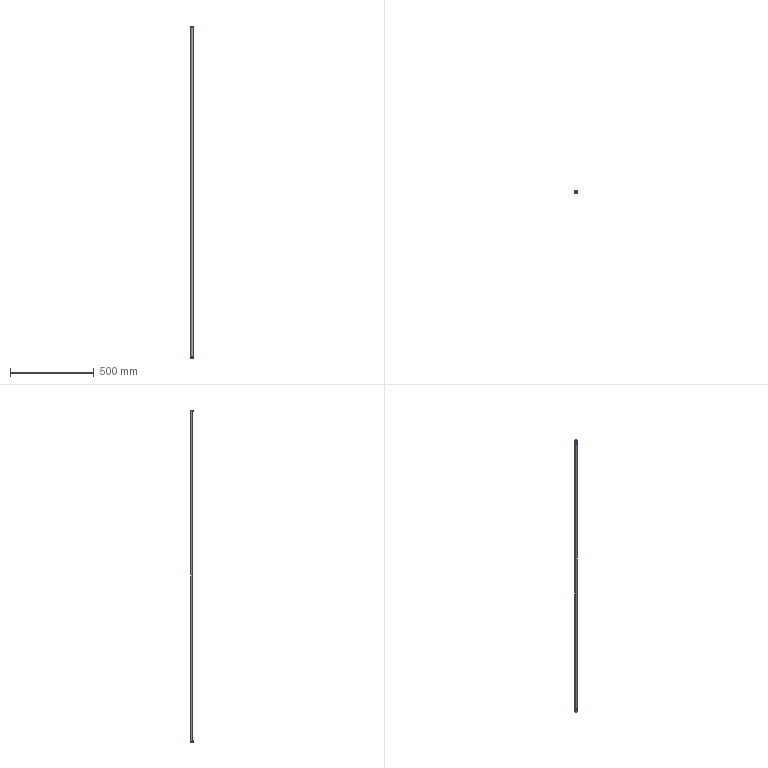Part | STEP file | X77-02003 | 1 solid | 32 faces | box 16 x 16 x 1981 mm | volume 394354 mm3 | plane 12 | cylinder 10 | cone 10 | commonest cylinder face diameters 8.8 x4 10 x4 16 x2
STEP:
#1=CARTESIAN_POINT('',(264.017,-37.994,1961.));
#2=VERTEX_POINT('',#1);
#3=CARTESIAN_POINT('',(274.017,-37.994,1961.));
#4=VERTEX_POINT('',#3);
#5=CARTESIAN_POINT('',(269.017,-37.994,1961.));
#6=DIRECTION('',(0.,0.,1.));
#7=DIRECTION('',(1.,0.,0.));
#8=AXIS2_PLACEMENT_3D('',#5,#6,#7);
#9=CIRCLE('',#8,5.);
#10=EDGE_CURVE('',#2,#4,#9,.T.);
#11=ORIENTED_EDGE('',*,*,#10,.F.);
#12=CARTESIAN_POINT('',(264.017,-37.994,1981.));
#13=VERTEX_POINT('',#12);
#14=CARTESIAN_POINT('',(264.017,-37.994,1981.));
#15=DIRECTION('',(0.,0.,1.));
#16=VECTOR('',#15,1000.);
#17=LINE('',#14,#16);
#18=EDGE_CURVE('',#2,#13,#17,.T.);
#19=ORIENTED_EDGE('',*,*,#18,.T.);
#20=CARTESIAN_POINT('',(274.017,-37.994,1981.));
#21=VERTEX_POINT('',#20);
#22=CARTESIAN_POINT('',(269.017,-37.994,1981.));
#23=DIRECTION('',(0.,0.,1.));
#24=DIRECTION('',(1.,0.,0.));
#25=AXIS2_PLACEMENT_3D('',#22,#23,#24);
#26=CIRCLE('',#25,5.);
#27=EDGE_CURVE('',#13,#21,#26,.T.);
#28=ORIENTED_EDGE('',*,*,#27,.T.);
#29=CARTESIAN_POINT('',(274.017,-37.994,1981.));
#30=DIRECTION('',(0.,0.,1.));
#31=VECTOR('',#30,1000.);
#32=LINE('',#29,#31);
#33=EDGE_CURVE('',#4,#21,#32,.T.);
#34=ORIENTED_EDGE('',*,*,#33,.F.);
#35=EDGE_LOOP('',(#11,#19,#28,#34));
#36=FACE_OUTER_BOUND('',#35,.T.);
#37=CARTESIAN_POINT('',(269.017,-37.994,1981.));
#38=DIRECTION('',(0.,0.,1.));
#39=DIRECTION('',(1.,0.,0.));
#40=AXIS2_PLACEMENT_3D('',#37,#38,#39);
#41=CYLINDRICAL_SURFACE('',#40,5.);
#42=ADVANCED_FACE('',(#36),#41,.F.);
#43=CARTESIAN_POINT('',(264.617,-37.994,1957.25));
#44=VERTEX_POINT('',#43);
#45=CARTESIAN_POINT('',(273.417,-37.994,1957.25));
#46=VERTEX_POINT('',#45);
#47=CARTESIAN_POINT('',(269.017,-37.994,1957.25));
#48=DIRECTION('',(0.,0.,1.));
#49=DIRECTION('',(1.,0.,0.));
#50=AXIS2_PLACEMENT_3D('',#47,#48,#49);
#51=CIRCLE('',#50,4.4);
#52=EDGE_CURVE('',#44,#46,#51,.T.);
#53=ORIENTED_EDGE('',*,*,#52,.F.);
#54=CARTESIAN_POINT('',(264.617,-37.994,1961.));
#55=VERTEX_POINT('',#54);
#56=CARTESIAN_POINT('',(264.617,-37.994,1981.));
#57=DIRECTION('',(0.,0.,1.));
#58=VECTOR('',#57,1000.);
#59=LINE('',#56,#58);
#60=EDGE_CURVE('',#44,#55,#59,.T.);
#61=ORIENTED_EDGE('',*,*,#60,.T.);
#62=CARTESIAN_POINT('',(273.417,-37.994,1961.));
#63=VERTEX_POINT('',#62);
#64=CARTESIAN_POINT('',(269.017,-37.994,1961.));
#65=DIRECTION('',(0.,0.,1.));
#66=DIRECTION('',(1.,0.,0.));
#67=AXIS2_PLACEMENT_3D('',#64,#65,#66);
#68=CIRCLE('',#67,4.4);
#69=EDGE_CURVE('',#55,#63,#68,.T.);
#70=ORIENTED_EDGE('',*,*,#69,.T.);
#71=CARTESIAN_POINT('',(273.417,-37.994,1981.));
#72=DIRECTION('',(0.,0.,1.));
#73=VECTOR('',#72,1000.);
#74=LINE('',#71,#73);
#75=EDGE_CURVE('',#46,#63,#74,.T.);
#76=ORIENTED_EDGE('',*,*,#75,.F.);
#77=EDGE_LOOP('',(#53,#61,#70,#76));
#78=FACE_OUTER_BOUND('',#77,.T.);
#79=CARTESIAN_POINT('',(269.017,-37.994,1981.));
#80=DIRECTION('',(0.,0.,1.));
#81=DIRECTION('',(1.,0.,0.));
#82=AXIS2_PLACEMENT_3D('',#79,#80,#81);
#83=CYLINDRICAL_SURFACE('',#82,4.4);
#84=ADVANCED_FACE('',(#78),#83,.F.);
#85=CARTESIAN_POINT('',(269.017,-37.994,1954.606));
#86=VERTEX_POINT('',#85);
#87=CARTESIAN_POINT('',(273.417,-37.994,1957.25));
#88=DIRECTION('',(0.8572,0.,0.515));
#89=VECTOR('',#88,1000.);
#90=LINE('',#87,#89);
#91=EDGE_CURVE('',#86,#46,#90,.T.);
#92=ORIENTED_EDGE('',*,*,#91,.F.);
#93=CARTESIAN_POINT('',(264.617,-37.994,1957.25));
#94=DIRECTION('',(-0.8572,0.,0.515));
#95=VECTOR('',#94,1000.);
#96=LINE('',#93,#95);
#97=EDGE_CURVE('',#86,#44,#96,.T.);
#98=ORIENTED_EDGE('',*,*,#97,.T.);
#99=ORIENTED_EDGE('',*,*,#52,.T.);
#100=EDGE_LOOP('',(#92,#98,#99));
#101=FACE_OUTER_BOUND('',#100,.T.);
#102=CARTESIAN_POINT('',(269.017,-37.994,1957.25));
#103=DIRECTION('',(0.,0.,1.));
#104=DIRECTION('',(1.,0.,0.));
#105=AXIS2_PLACEMENT_3D('',#102,#103,#104);
#106=CONICAL_SURFACE('',#105,4.4,1.03);
#107=ADVANCED_FACE('',(#101),#106,.F.);
#108=CARTESIAN_POINT('',(274.017,-37.994,20.));
#109=VERTEX_POINT('',#108);
#110=CARTESIAN_POINT('',(264.017,-37.994,20.));
#111=VERTEX_POINT('',#110);
#112=CARTESIAN_POINT('',(269.017,-37.994,20.));
#113=DIRECTION('',(0.,0.,-1.));
#114=DIRECTION('',(-1.,0.,0.));
#115=AXIS2_PLACEMENT_3D('',#112,#113,#114);
#116=CIRCLE('',#115,5.);
#117=EDGE_CURVE('',#109,#111,#116,.T.);
#118=ORIENTED_EDGE('',*,*,#117,.F.);
#119=CARTESIAN_POINT('',(274.017,-37.994,0.));
#120=VERTEX_POINT('',#119);
#121=CARTESIAN_POINT('',(274.017,-37.994,0.));
#122=DIRECTION('',(0.,0.,-1.));
#123=VECTOR('',#122,1000.);
#124=LINE('',#121,#123);
#125=EDGE_CURVE('',#109,#120,#124,.T.);
#126=ORIENTED_EDGE('',*,*,#125,.T.);
#127=CARTESIAN_POINT('',(264.017,-37.994,0.));
#128=VERTEX_POINT('',#127);
#129=CARTESIAN_POINT('',(269.017,-37.994,0.));
#130=DIRECTION('',(0.,0.,-1.));
#131=DIRECTION('',(-1.,0.,0.));
#132=AXIS2_PLACEMENT_3D('',#129,#130,#131);
#133=CIRCLE('',#132,5.);
#134=EDGE_CURVE('',#120,#128,#133,.T.);
#135=ORIENTED_EDGE('',*,*,#134,.T.);
#136=CARTESIAN_POINT('',(264.017,-37.994,0.));
#137=DIRECTION('',(0.,0.,-1.));
#138=VECTOR('',#137,1000.);
#139=LINE('',#136,#138);
#140=EDGE_CURVE('',#111,#128,#139,.T.);
#141=ORIENTED_EDGE('',*,*,#140,.F.);
#142=EDGE_LOOP('',(#118,#126,#135,#141));
#143=FACE_OUTER_BOUND('',#142,.T.);
#144=CARTESIAN_POINT('',(269.017,-37.994,0.));
#145=DIRECTION('',(0.,0.,-1.));
#146=DIRECTION('',(-1.,0.,0.));
#147=AXIS2_PLACEMENT_3D('',#144,#145,#146);
#148=CYLINDRICAL_SURFACE('',#147,5.);
#149=ADVANCED_FACE('',(#143),#148,.F.);
#150=CARTESIAN_POINT('',(273.417,-37.994,23.75));
#151=VERTEX_POINT('',#150);
#152=CARTESIAN_POINT('',(264.617,-37.994,23.75));
#153=VERTEX_POINT('',#152);
#154=CARTESIAN_POINT('',(269.017,-37.994,23.75));
#155=DIRECTION('',(0.,0.,-1.));
#156=DIRECTION('',(-1.,0.,0.));
#157=AXIS2_PLACEMENT_3D('',#154,#155,#156);
#158=CIRCLE('',#157,4.4);
#159=EDGE_CURVE('',#151,#153,#158,.T.);
#160=ORIENTED_EDGE('',*,*,#159,.F.);
#161=CARTESIAN_POINT('',(273.417,-37.994,20.));
#162=VERTEX_POINT('',#161);
#163=CARTESIAN_POINT('',(273.417,-37.994,0.));
#164=DIRECTION('',(0.,0.,-1.));
#165=VECTOR('',#164,1000.);
#166=LINE('',#163,#165);
#167=EDGE_CURVE('',#151,#162,#166,.T.);
#168=ORIENTED_EDGE('',*,*,#167,.T.);
#169=CARTESIAN_POINT('',(264.617,-37.994,20.));
#170=VERTEX_POINT('',#169);
#171=CARTESIAN_POINT('',(269.017,-37.994,20.));
#172=DIRECTION('',(0.,0.,-1.));
#173=DIRECTION('',(-1.,0.,0.));
#174=AXIS2_PLACEMENT_3D('',#171,#172,#173);
#175=CIRCLE('',#174,4.4);
#176=EDGE_CURVE('',#162,#170,#175,.T.);
#177=ORIENTED_EDGE('',*,*,#176,.T.);
#178=CARTESIAN_POINT('',(264.617,-37.994,0.));
#179=DIRECTION('',(0.,0.,-1.));
#180=VECTOR('',#179,1000.);
#181=LINE('',#178,#180);
#182=EDGE_CURVE('',#153,#170,#181,.T.);
#183=ORIENTED_EDGE('',*,*,#182,.F.);
#184=EDGE_LOOP('',(#160,#168,#177,#183));
#185=FACE_OUTER_BOUND('',#184,.T.);
#186=CARTESIAN_POINT('',(269.017,-37.994,0.));
#187=DIRECTION('',(0.,0.,-1.));
#188=DIRECTION('',(-1.,0.,0.));
#189=AXIS2_PLACEMENT_3D('',#186,#187,#188);
#190=CYLINDRICAL_SURFACE('',#189,4.4);
#191=ADVANCED_FACE('',(#185),#190,.F.);
#192=CARTESIAN_POINT('',(269.017,-37.994,26.394));
#193=VERTEX_POINT('',#192);
#194=CARTESIAN_POINT('',(264.617,-37.994,23.75));
#195=DIRECTION('',(-0.8572,0.,-0.515));
#196=VECTOR('',#195,1000.);
#197=LINE('',#194,#196);
#198=EDGE_CURVE('',#193,#153,#197,.T.);
#199=ORIENTED_EDGE('',*,*,#198,.F.);
#200=CARTESIAN_POINT('',(273.417,-37.994,23.75));
#201=DIRECTION('',(0.8572,0.,-0.515));
#202=VECTOR('',#201,1000.);
#203=LINE('',#200,#202);
#204=EDGE_CURVE('',#193,#151,#203,.T.);
#205=ORIENTED_EDGE('',*,*,#204,.T.);
#206=ORIENTED_EDGE('',*,*,#159,.T.);
#207=EDGE_LOOP('',(#199,#205,#206));
#208=FACE_OUTER_BOUND('',#207,.T.);
#209=CARTESIAN_POINT('',(269.017,-37.994,23.75));
#210=DIRECTION('',(0.,0.,-1.));
#211=DIRECTION('',(-1.,0.,0.));
#212=AXIS2_PLACEMENT_3D('',#209,#210,#211);
#213=CONICAL_SURFACE('',#212,4.4,1.03);
#214=ADVANCED_FACE('',(#208),#213,.F.);
#215=CARTESIAN_POINT('',(276.017,-37.994,0.));
#216=VERTEX_POINT('',#215);
#217=CARTESIAN_POINT('',(269.017,-44.994,0.));
#218=VERTEX_POINT('',#217);
#219=CARTESIAN_POINT('',(269.017,-37.994,0.));
#220=DIRECTION('',(0.,0.,-1.));
#221=DIRECTION('',(1.,0.,0.));
#222=AXIS2_PLACEMENT_3D('',#219,#220,#221);
#223=CIRCLE('',#222,7.);
#224=EDGE_CURVE('',#216,#218,#223,.T.);
#225=ORIENTED_EDGE('',*,*,#224,.F.);
#226=CARTESIAN_POINT('',(277.017,-37.994,1.));
#227=VERTEX_POINT('',#226);
#228=CARTESIAN_POINT('',(277.017,-37.994,1.));
#229=DIRECTION('',(0.7071,0.,0.7071));
#230=VECTOR('',#229,1000.);
#231=LINE('',#228,#230);
#232=EDGE_CURVE('',#216,#227,#231,.T.);
#233=ORIENTED_EDGE('',*,*,#232,.T.);
#234=CARTESIAN_POINT('',(272.89,-44.994,1.));
#235=VERTEX_POINT('',#234);
#236=CARTESIAN_POINT('',(269.017,-37.994,1.));
#237=DIRECTION('',(0.,0.,1.));
#238=DIRECTION('',(1.,0.,0.));
#239=AXIS2_PLACEMENT_3D('',#236,#237,#238);
#240=CIRCLE('',#239,8.);
#241=EDGE_CURVE('',#235,#227,#240,.T.);
#242=ORIENTED_EDGE('',*,*,#241,.F.);
#243=CARTESIAN_POINT('',(272.89,-44.994,1.));
#244=CARTESIAN_POINT('',(272.59,-44.994,0.8546));
#245=CARTESIAN_POINT('',(272.284,-44.994,0.7192));
#246=CARTESIAN_POINT('',(271.656,-44.994,0.4753));
#247=CARTESIAN_POINT('',(271.334,-44.994,0.3667));
#248=CARTESIAN_POINT('',(270.685,-44.994,0.1892));
#249=CARTESIAN_POINT('',(270.357,-44.994,0.1196));
#250=CARTESIAN_POINT('',(269.694,-44.994,0.02493));
#251=CARTESIAN_POINT('',(269.357,-44.994,0.));
#252=CARTESIAN_POINT('',(269.017,-44.994,0.));
#253=B_SPLINE_CURVE_WITH_KNOTS('',3,(#243,#244,#245,#246,#247,#248,#249,#250,#251,#252),.UNSPECIFIED.,.F.,.F.,(4,2,2,2,4),(0.004369,0.005367,0.006366,0.007365,0.008364),.UNSPECIFIED.);
#254=EDGE_CURVE('',#235,#218,#253,.T.);
#255=ORIENTED_EDGE('',*,*,#254,.T.);
#256=EDGE_LOOP('',(#225,#233,#242,#255));
#257=FACE_OUTER_BOUND('',#256,.T.);
#258=CARTESIAN_POINT('',(269.017,-37.994,1.));
#259=DIRECTION('',(0.,0.,1.));
#260=DIRECTION('',(1.,0.,0.));
#261=AXIS2_PLACEMENT_3D('',#258,#259,#260);
#262=CONICAL_SURFACE('',#261,8.,0.7854);
#263=ADVANCED_FACE('',(#257),#262,.T.);
#264=CARTESIAN_POINT('',(262.017,-37.994,1981.));
#265=VERTEX_POINT('',#264);
#266=CARTESIAN_POINT('',(269.017,-44.994,1981.));
#267=VERTEX_POINT('',#266);
#268=CARTESIAN_POINT('',(269.017,-37.994,1981.));
#269=DIRECTION('',(0.,0.,1.));
#270=DIRECTION('',(1.,0.,0.));
#271=AXIS2_PLACEMENT_3D('',#268,#269,#270);
#272=CIRCLE('',#271,7.);
#273=EDGE_CURVE('',#265,#267,#272,.T.);
#274=ORIENTED_EDGE('',*,*,#273,.F.);
#275=CARTESIAN_POINT('',(261.017,-37.994,1980.));
#276=VERTEX_POINT('',#275);
#277=CARTESIAN_POINT('',(262.017,-37.994,1981.));
#278=DIRECTION('',(-0.7071,0.,-0.7071));
#279=VECTOR('',#278,1000.);
#280=LINE('',#277,#279);
#281=EDGE_CURVE('',#265,#276,#280,.T.);
#282=ORIENTED_EDGE('',*,*,#281,.T.);
#283=CARTESIAN_POINT('',(265.144,-44.994,1980.));
#284=VERTEX_POINT('',#283);
#285=CARTESIAN_POINT('',(269.017,-37.994,1980.));
#286=DIRECTION('',(0.,0.,-1.));
#287=DIRECTION('',(1.,0.,0.));
#288=AXIS2_PLACEMENT_3D('',#285,#286,#287);
#289=CIRCLE('',#288,8.);
#290=EDGE_CURVE('',#284,#276,#289,.T.);
#291=ORIENTED_EDGE('',*,*,#290,.F.);
#292=CARTESIAN_POINT('',(265.144,-44.994,1980.));
#293=CARTESIAN_POINT('',(265.741,-44.994,1980.289));
#294=CARTESIAN_POINT('',(266.361,-44.994,1980.54));
#295=CARTESIAN_POINT('',(267.671,-44.994,1980.9));
#296=CARTESIAN_POINT('',(268.337,-44.994,1981.));
#297=CARTESIAN_POINT('',(269.017,-44.994,1981.));
#298=B_SPLINE_CURVE_WITH_KNOTS('',3,(#292,#293,#294,#295,#296,#297),.UNSPECIFIED.,.F.,.F.,(4,2,4),(0.02013,0.02213,0.02413),.UNSPECIFIED.);
#299=EDGE_CURVE('',#284,#267,#298,.T.);
#300=ORIENTED_EDGE('',*,*,#299,.T.);
#301=EDGE_LOOP('',(#274,#282,#291,#300));
#302=FACE_OUTER_BOUND('',#301,.T.);
#303=CARTESIAN_POINT('',(269.017,-37.994,1981.));
#304=DIRECTION('',(0.,0.,-1.));
#305=DIRECTION('',(-1.,0.,0.));
#306=AXIS2_PLACEMENT_3D('',#303,#304,#305);
#307=CONICAL_SURFACE('',#306,7.,0.7854);
#308=ADVANCED_FACE('',(#302),#307,.T.);
#309=CARTESIAN_POINT('',(272.89,-30.994,1980.));
#310=VERTEX_POINT('',#309);
#311=CARTESIAN_POINT('',(277.017,-37.994,1980.));
#312=VERTEX_POINT('',#311);
#313=CARTESIAN_POINT('',(269.017,-37.994,1980.));
#314=DIRECTION('',(0.,0.,-1.));
#315=DIRECTION('',(1.,0.,0.));
#316=AXIS2_PLACEMENT_3D('',#313,#314,#315);
#317=CIRCLE('',#316,8.);
#318=EDGE_CURVE('',#310,#312,#317,.T.);
#319=ORIENTED_EDGE('',*,*,#318,.T.);
#320=CARTESIAN_POINT('',(277.017,-37.994,1981.));
#321=DIRECTION('',(0.,0.,-1.));
#322=VECTOR('',#321,1000.);
#323=LINE('',#320,#322);
#324=EDGE_CURVE('',#312,#227,#323,.T.);
#325=ORIENTED_EDGE('',*,*,#324,.T.);
#326=CARTESIAN_POINT('',(272.89,-30.994,1.));
#327=VERTEX_POINT('',#326);
#328=CARTESIAN_POINT('',(269.017,-37.994,1.));
#329=DIRECTION('',(0.,0.,1.));
#330=DIRECTION('',(1.,0.,0.));
#331=AXIS2_PLACEMENT_3D('',#328,#329,#330);
#332=CIRCLE('',#331,8.);
#333=EDGE_CURVE('',#227,#327,#332,.T.);
#334=ORIENTED_EDGE('',*,*,#333,.T.);
#335=CARTESIAN_POINT('',(272.89,-30.994,10.));
#336=VERTEX_POINT('',#335);
#337=CARTESIAN_POINT('',(272.89,-30.994,1981.));
#338=DIRECTION('',(0.,0.,-1.));
#339=VECTOR('',#338,1000.);
#340=LINE('',#337,#339);
#341=EDGE_CURVE('',#336,#327,#340,.T.);
#342=ORIENTED_EDGE('',*,*,#341,.F.);
#343=CARTESIAN_POINT('',(265.144,-30.994,10.));
#344=VERTEX_POINT('',#343);
#345=CARTESIAN_POINT('',(269.017,-37.994,10.));
#346=DIRECTION('',(0.,0.,-1.));
#347=DIRECTION('',(-1.,0.,0.));
#348=AXIS2_PLACEMENT_3D('',#345,#346,#347);
#349=CIRCLE('',#348,8.);
#350=EDGE_CURVE('',#344,#336,#349,.T.);
#351=ORIENTED_EDGE('',*,*,#350,.F.);
#352=CARTESIAN_POINT('',(265.144,-30.994,1.));
#353=VERTEX_POINT('',#352);
#354=CARTESIAN_POINT('',(265.144,-30.994,1981.));
#355=DIRECTION('',(0.,0.,1.));
#356=VECTOR('',#355,1000.);
#357=LINE('',#354,#356);
#358=EDGE_CURVE('',#353,#344,#357,.T.);
#359=ORIENTED_EDGE('',*,*,#358,.F.);
#360=CARTESIAN_POINT('',(261.017,-37.994,1.));
#361=VERTEX_POINT('',#360);
#362=CARTESIAN_POINT('',(269.017,-37.994,1.));
#363=DIRECTION('',(0.,0.,1.));
#364=DIRECTION('',(1.,0.,0.));
#365=AXIS2_PLACEMENT_3D('',#362,#363,#364);
#366=CIRCLE('',#365,8.);
#367=EDGE_CURVE('',#353,#361,#366,.T.);
#368=ORIENTED_EDGE('',*,*,#367,.T.);
#369=CARTESIAN_POINT('',(261.017,-37.994,1981.));
#370=DIRECTION('',(0.,0.,-1.));
#371=VECTOR('',#370,1000.);
#372=LINE('',#369,#371);
#373=EDGE_CURVE('',#276,#361,#372,.T.);
#374=ORIENTED_EDGE('',*,*,#373,.F.);
#375=CARTESIAN_POINT('',(265.144,-30.994,1980.));
#376=VERTEX_POINT('',#375);
#377=CARTESIAN_POINT('',(269.017,-37.994,1980.));
#378=DIRECTION('',(0.,0.,-1.));
#379=DIRECTION('',(1.,0.,0.));
#380=AXIS2_PLACEMENT_3D('',#377,#378,#379);
#381=CIRCLE('',#380,8.);
#382=EDGE_CURVE('',#276,#376,#381,.T.);
#383=ORIENTED_EDGE('',*,*,#382,.T.);
#384=CARTESIAN_POINT('',(265.144,-30.994,1971.));
#385=VERTEX_POINT('',#384);
#386=CARTESIAN_POINT('',(265.144,-30.994,1981.));
#387=DIRECTION('',(0.,0.,1.));
#388=VECTOR('',#387,1000.);
#389=LINE('',#386,#388);
#390=EDGE_CURVE('',#385,#376,#389,.T.);
#391=ORIENTED_EDGE('',*,*,#390,.F.);
#392=CARTESIAN_POINT('',(272.89,-30.994,1971.));
#393=VERTEX_POINT('',#392);
#394=CARTESIAN_POINT('',(269.017,-37.994,1971.));
#395=DIRECTION('',(0.,0.,1.));
#396=DIRECTION('',(1.,0.,0.));
#397=AXIS2_PLACEMENT_3D('',#394,#395,#396);
#398=CIRCLE('',#397,8.);
#399=EDGE_CURVE('',#393,#385,#398,.T.);
#400=ORIENTED_EDGE('',*,*,#399,.F.);
#401=CARTESIAN_POINT('',(272.89,-30.994,1981.));
#402=DIRECTION('',(0.,0.,-1.));
#403=VECTOR('',#402,1000.);
#404=LINE('',#401,#403);
#405=EDGE_CURVE('',#310,#393,#404,.T.);
#406=ORIENTED_EDGE('',*,*,#405,.F.);
#407=EDGE_LOOP('',(#319,#325,#334,#342,#351,#359,#368,#374,#383,#391,#400,#406));
#408=FACE_OUTER_BOUND('',#407,.T.);
#409=CARTESIAN_POINT('',(269.017,-37.994,1981.));
#410=DIRECTION('',(0.,0.,-1.));
#411=DIRECTION('',(-1.,0.,0.));
#412=AXIS2_PLACEMENT_3D('',#409,#410,#411);
#413=CYLINDRICAL_SURFACE('',#412,8.);
#414=ADVANCED_FACE('',(#408),#413,.T.);
#415=ORIENTED_EDGE('',*,*,#324,.F.);
#416=CARTESIAN_POINT('',(272.89,-44.994,1980.));
#417=VERTEX_POINT('',#416);
#418=CARTESIAN_POINT('',(269.017,-37.994,1980.));
#419=DIRECTION('',(0.,0.,-1.));
#420=DIRECTION('',(1.,0.,0.));
#421=AXIS2_PLACEMENT_3D('',#418,#419,#420);
#422=CIRCLE('',#421,8.);
#423=EDGE_CURVE('',#312,#417,#422,.T.);
#424=ORIENTED_EDGE('',*,*,#423,.T.);
#425=CARTESIAN_POINT('',(272.89,-44.994,1971.));
#426=VERTEX_POINT('',#425);
#427=CARTESIAN_POINT('',(272.89,-44.994,1981.));
#428=DIRECTION('',(0.,0.,1.));
#429=VECTOR('',#428,1000.);
#430=LINE('',#427,#429);
#431=EDGE_CURVE('',#426,#417,#430,.T.);
#432=ORIENTED_EDGE('',*,*,#431,.F.);
#433=CARTESIAN_POINT('',(265.144,-44.994,1971.));
#434=VERTEX_POINT('',#433);
#435=CARTESIAN_POINT('',(269.017,-37.994,1971.));
#436=DIRECTION('',(0.,0.,1.));
#437=DIRECTION('',(1.,0.,0.));
#438=AXIS2_PLACEMENT_3D('',#435,#436,#437);
#439=CIRCLE('',#438,8.);
#440=EDGE_CURVE('',#434,#426,#439,.T.);
#441=ORIENTED_EDGE('',*,*,#440,.F.);
#442=CARTESIAN_POINT('',(265.144,-44.994,1981.));
#443=DIRECTION('',(0.,0.,-1.));
#444=VECTOR('',#443,1000.);
#445=LINE('',#442,#444);
#446=EDGE_CURVE('',#284,#434,#445,.T.);
#447=ORIENTED_EDGE('',*,*,#446,.F.);
#448=ORIENTED_EDGE('',*,*,#290,.T.);
#449=ORIENTED_EDGE('',*,*,#373,.T.);
#450=CARTESIAN_POINT('',(265.144,-44.994,1.));
#451=VERTEX_POINT('',#450);
#452=CARTESIAN_POINT('',(269.017,-37.994,1.));
#453=DIRECTION('',(0.,0.,1.));
#454=DIRECTION('',(1.,0.,0.));
#455=AXIS2_PLACEMENT_3D('',#452,#453,#454);
#456=CIRCLE('',#455,8.);
#457=EDGE_CURVE('',#361,#451,#456,.T.);
#458=ORIENTED_EDGE('',*,*,#457,.T.);
#459=CARTESIAN_POINT('',(265.144,-44.994,10.));
#460=VERTEX_POINT('',#459);
#461=CARTESIAN_POINT('',(265.144,-44.994,1981.));
#462=DIRECTION('',(0.,0.,-1.));
#463=VECTOR('',#462,1000.);
#464=LINE('',#461,#463);
#465=EDGE_CURVE('',#460,#451,#464,.T.);
#466=ORIENTED_EDGE('',*,*,#465,.F.);
#467=CARTESIAN_POINT('',(272.89,-44.994,10.));
#468=VERTEX_POINT('',#467);
#469=CARTESIAN_POINT('',(269.017,-37.994,10.));
#470=DIRECTION('',(0.,0.,-1.));
#471=DIRECTION('',(-1.,0.,0.));
#472=AXIS2_PLACEMENT_3D('',#469,#470,#471);
#473=CIRCLE('',#472,8.);
#474=EDGE_CURVE('',#468,#460,#473,.T.);
#475=ORIENTED_EDGE('',*,*,#474,.F.);
#476=CARTESIAN_POINT('',(272.89,-44.994,1981.));
#477=DIRECTION('',(0.,0.,1.));
#478=VECTOR('',#477,1000.);
#479=LINE('',#476,#478);
#480=EDGE_CURVE('',#235,#468,#479,.T.);
#481=ORIENTED_EDGE('',*,*,#480,.F.);
#482=ORIENTED_EDGE('',*,*,#241,.T.);
#483=EDGE_LOOP('',(#415,#424,#432,#441,#447,#448,#449,#458,#466,#475,#481,#482));
#484=FACE_OUTER_BOUND('',#483,.T.);
#485=CARTESIAN_POINT('',(269.017,-37.994,1981.));
#486=DIRECTION('',(0.,0.,-1.));
#487=DIRECTION('',(-1.,0.,0.));
#488=AXIS2_PLACEMENT_3D('',#485,#486,#487);
#489=CYLINDRICAL_SURFACE('',#488,8.);
#490=ADVANCED_FACE('',(#484),#489,.T.);
#491=ORIENTED_EDGE('',*,*,#281,.F.);
#492=CARTESIAN_POINT('',(269.017,-30.994,1981.));
#493=VERTEX_POINT('',#492);
#494=CARTESIAN_POINT('',(269.017,-37.994,1981.));
#495=DIRECTION('',(0.,0.,1.));
#496=DIRECTION('',(1.,0.,0.));
#497=AXIS2_PLACEMENT_3D('',#494,#495,#496);
#498=CIRCLE('',#497,7.);
#499=EDGE_CURVE('',#493,#265,#498,.T.);
#500=ORIENTED_EDGE('',*,*,#499,.F.);
#501=CARTESIAN_POINT('',(269.017,-30.994,1981.));
#502=CARTESIAN_POINT('',(268.337,-30.994,1981.));
#503=CARTESIAN_POINT('',(267.671,-30.994,1980.9));
#504=CARTESIAN_POINT('',(266.361,-30.994,1980.54));
#505=CARTESIAN_POINT('',(265.741,-30.994,1980.289));
#506=CARTESIAN_POINT('',(265.144,-30.994,1980.));
#507=B_SPLINE_CURVE_WITH_KNOTS('',3,(#501,#502,#503,#504,#505,#506),.UNSPECIFIED.,.F.,.F.,(4,2,4),(0.008364,0.01037,0.01237),.UNSPECIFIED.);
#508=EDGE_CURVE('',#493,#376,#507,.T.);
#509=ORIENTED_EDGE('',*,*,#508,.T.);
#510=ORIENTED_EDGE('',*,*,#382,.F.);
#511=EDGE_LOOP('',(#491,#500,#509,#510));
#512=FACE_OUTER_BOUND('',#511,.T.);
#513=CARTESIAN_POINT('',(269.017,-37.994,1981.));
#514=DIRECTION('',(0.,0.,-1.));
#515=DIRECTION('',(-1.,0.,0.));
#516=AXIS2_PLACEMENT_3D('',#513,#514,#515);
#517=CONICAL_SURFACE('',#516,7.,0.7854);
#518=ADVANCED_FACE('',(#512),#517,.T.);
#519=CARTESIAN_POINT('',(269.017,-37.994,1981.));
#520=DIRECTION('',(0.,0.,1.));
#521=DIRECTION('',(1.,0.,0.));
#522=AXIS2_PLACEMENT_3D('',#519,#520,#521);
#523=CIRCLE('',#522,7.);
#524=EDGE_CURVE('',#267,#493,#523,.T.);
#525=ORIENTED_EDGE('',*,*,#524,.F.);
#526=CARTESIAN_POINT('',(269.017,-44.994,1981.));
#527=CARTESIAN_POINT('',(269.357,-44.994,1981.));
#528=CARTESIAN_POINT('',(269.694,-44.994,1980.975));
#529=CARTESIAN_POINT('',(270.357,-44.994,1980.88));
#530=CARTESIAN_POINT('',(270.685,-44.994,1980.811));
#531=CARTESIAN_POINT('',(271.334,-44.994,1980.633));
#532=CARTESIAN_POINT('',(271.656,-44.994,1980.525));
#533=CARTESIAN_POINT('',(272.284,-44.994,1980.281));
#534=CARTESIAN_POINT('',(272.59,-44.994,1980.145));
#535=CARTESIAN_POINT('',(272.89,-44.994,1980.));
#536=B_SPLINE_CURVE_WITH_KNOTS('',3,(#526,#527,#528,#529,#530,#531,#532,#533,#534,#535),.UNSPECIFIED.,.F.,.F.,(4,2,2,2,4),(0.02413,0.02513,0.02612,0.02712,0.02812),.UNSPECIFIED.);
#537=EDGE_CURVE('',#267,#417,#536,.T.);
#538=ORIENTED_EDGE('',*,*,#537,.T.);
#539=ORIENTED_EDGE('',*,*,#423,.F.);
#540=ORIENTED_EDGE('',*,*,#318,.F.);
#541=CARTESIAN_POINT('',(272.89,-30.994,1980.));
#542=CARTESIAN_POINT('',(272.59,-30.994,1980.145));
#543=CARTESIAN_POINT('',(272.284,-30.994,1980.281));
#544=CARTESIAN_POINT('',(271.656,-30.994,1980.525));
#545=CARTESIAN_POINT('',(271.334,-30.994,1980.633));
#546=CARTESIAN_POINT('',(270.685,-30.994,1980.811));
#547=CARTESIAN_POINT('',(270.357,-30.994,1980.88));
#548=CARTESIAN_POINT('',(269.694,-30.994,1980.975));
#549=CARTESIAN_POINT('',(269.357,-30.994,1981.));
#550=CARTESIAN_POINT('',(269.017,-30.994,1981.));
#551=B_SPLINE_CURVE_WITH_KNOTS('',3,(#541,#542,#543,#544,#545,#546,#547,#548,#549,#550),.UNSPECIFIED.,.F.,.F.,(4,2,2,2,4),(0.004369,0.005367,0.006366,0.007365,0.008364),.UNSPECIFIED.);
#552=EDGE_CURVE('',#310,#493,#551,.T.);
#553=ORIENTED_EDGE('',*,*,#552,.T.);
#554=EDGE_LOOP('',(#525,#538,#539,#540,#553));
#555=FACE_OUTER_BOUND('',#554,.T.);
#556=CARTESIAN_POINT('',(269.017,-37.994,1981.));
#557=DIRECTION('',(0.,0.,-1.));
#558=DIRECTION('',(-1.,0.,0.));
#559=AXIS2_PLACEMENT_3D('',#556,#557,#558);
#560=CONICAL_SURFACE('',#559,7.,0.7854);
#561=ADVANCED_FACE('',(#555),#560,.T.);
#562=ORIENTED_EDGE('',*,*,#232,.F.);
#563=CARTESIAN_POINT('',(269.017,-30.994,0.));
#564=VERTEX_POINT('',#563);
#565=CARTESIAN_POINT('',(269.017,-37.994,0.));
#566=DIRECTION('',(0.,0.,-1.));
#567=DIRECTION('',(1.,0.,0.));
#568=AXIS2_PLACEMENT_3D('',#565,#566,#567);
#569=CIRCLE('',#568,7.);
#570=EDGE_CURVE('',#564,#216,#569,.T.);
#571=ORIENTED_EDGE('',*,*,#570,.F.);
#572=CARTESIAN_POINT('',(269.017,-30.994,0.));
#573=CARTESIAN_POINT('',(269.357,-30.994,0.));
#574=CARTESIAN_POINT('',(269.694,-30.994,0.02493));
#575=CARTESIAN_POINT('',(270.357,-30.994,0.1196));
#576=CARTESIAN_POINT('',(270.685,-30.994,0.1892));
#577=CARTESIAN_POINT('',(271.334,-30.994,0.3667));
#578=CARTESIAN_POINT('',(271.656,-30.994,0.4753));
#579=CARTESIAN_POINT('',(272.284,-30.994,0.7192));
#580=CARTESIAN_POINT('',(272.59,-30.994,0.8546));
#581=CARTESIAN_POINT('',(272.89,-30.994,1.));
#582=B_SPLINE_CURVE_WITH_KNOTS('',3,(#572,#573,#574,#575,#576,#577,#578,#579,#580,#581),.UNSPECIFIED.,.F.,.F.,(4,2,2,2,4),(0.02413,0.02513,0.02612,0.02712,0.02812),.UNSPECIFIED.);
#583=EDGE_CURVE('',#564,#327,#582,.T.);
#584=ORIENTED_EDGE('',*,*,#583,.T.);
#585=ORIENTED_EDGE('',*,*,#333,.F.);
#586=EDGE_LOOP('',(#562,#571,#584,#585));
#587=FACE_OUTER_BOUND('',#586,.T.);
#588=CARTESIAN_POINT('',(269.017,-37.994,1.));
#589=DIRECTION('',(0.,0.,1.));
#590=DIRECTION('',(1.,0.,0.));
#591=AXIS2_PLACEMENT_3D('',#588,#589,#590);
#592=CONICAL_SURFACE('',#591,8.,0.7854);
#593=ADVANCED_FACE('',(#587),#592,.T.);
#594=CARTESIAN_POINT('',(269.017,-37.994,0.));
#595=DIRECTION('',(0.,0.,-1.));
#596=DIRECTION('',(1.,0.,0.));
#597=AXIS2_PLACEMENT_3D('',#594,#595,#596);
#598=CIRCLE('',#597,7.);
#599=EDGE_CURVE('',#218,#564,#598,.T.);
#600=ORIENTED_EDGE('',*,*,#599,.F.);
#601=CARTESIAN_POINT('',(269.017,-44.994,0.));
#602=CARTESIAN_POINT('',(268.337,-44.994,0.));
#603=CARTESIAN_POINT('',(267.671,-44.994,0.1004));
#604=CARTESIAN_POINT('',(266.361,-44.994,0.4605));
#605=CARTESIAN_POINT('',(265.741,-44.994,0.711));
#606=CARTESIAN_POINT('',(265.144,-44.994,1.));
#607=B_SPLINE_CURVE_WITH_KNOTS('',3,(#601,#602,#603,#604,#605,#606),.UNSPECIFIED.,.F.,.F.,(4,2,4),(0.008364,0.01037,0.01237),.UNSPECIFIED.);
#608=EDGE_CURVE('',#218,#451,#607,.T.);
#609=ORIENTED_EDGE('',*,*,#608,.T.);
#610=ORIENTED_EDGE('',*,*,#457,.F.);
#611=ORIENTED_EDGE('',*,*,#367,.F.);
#612=CARTESIAN_POINT('',(265.144,-30.994,1.));
#613=CARTESIAN_POINT('',(265.741,-30.994,0.711));
#614=CARTESIAN_POINT('',(266.361,-30.994,0.4605));
#615=CARTESIAN_POINT('',(267.671,-30.994,0.1004));
#616=CARTESIAN_POINT('',(268.337,-30.994,0.));
#617=CARTESIAN_POINT('',(269.017,-30.994,0.));
#618=B_SPLINE_CURVE_WITH_KNOTS('',3,(#612,#613,#614,#615,#616,#617),.UNSPECIFIED.,.F.,.F.,(4,2,4),(0.02013,0.02213,0.02413),.UNSPECIFIED.);
#619=EDGE_CURVE('',#353,#564,#618,.T.);
#620=ORIENTED_EDGE('',*,*,#619,.T.);
#621=EDGE_LOOP('',(#600,#609,#610,#611,#620));
#622=FACE_OUTER_BOUND('',#621,.T.);
#623=CARTESIAN_POINT('',(269.017,-37.994,1.));
#624=DIRECTION('',(0.,0.,1.));
#625=DIRECTION('',(1.,0.,0.));
#626=AXIS2_PLACEMENT_3D('',#623,#624,#625);
#627=CONICAL_SURFACE('',#626,8.,0.7854);
#628=ADVANCED_FACE('',(#622),#627,.T.);
#629=CARTESIAN_POINT('',(269.017,-37.994,1981.));
#630=DIRECTION('',(0.,0.,1.));
#631=DIRECTION('',(1.,0.,0.));
#632=AXIS2_PLACEMENT_3D('',#629,#630,#631);
#633=CIRCLE('',#632,5.);
#634=EDGE_CURVE('',#21,#13,#633,.T.);
#635=ORIENTED_EDGE('',*,*,#634,.F.);
#636=ORIENTED_EDGE('',*,*,#27,.F.);
#637=EDGE_LOOP('',(#635,#636));
#638=FACE_BOUND('',#637,.T.);
#639=ORIENTED_EDGE('',*,*,#499,.T.);
#640=ORIENTED_EDGE('',*,*,#273,.T.);
#641=ORIENTED_EDGE('',*,*,#524,.T.);
#642=EDGE_LOOP('',(#639,#640,#641));
#643=FACE_OUTER_BOUND('',#642,.T.);
#644=CARTESIAN_POINT('',(269.017,-37.994,1981.));
#645=DIRECTION('',(0.,0.,1.));
#646=DIRECTION('',(1.,0.,0.));
#647=AXIS2_PLACEMENT_3D('',#644,#645,#646);
#648=PLANE('',#647);
#649=ADVANCED_FACE('',(#638,#643),#648,.T.);
#650=CARTESIAN_POINT('',(269.017,-37.994,0.));
#651=DIRECTION('',(0.,0.,-1.));
#652=DIRECTION('',(-1.,0.,0.));
#653=AXIS2_PLACEMENT_3D('',#650,#651,#652);
#654=CIRCLE('',#653,5.);
#655=EDGE_CURVE('',#128,#120,#654,.T.);
#656=ORIENTED_EDGE('',*,*,#655,.F.);
#657=ORIENTED_EDGE('',*,*,#134,.F.);
#658=EDGE_LOOP('',(#656,#657));
#659=FACE_BOUND('',#658,.T.);
#660=ORIENTED_EDGE('',*,*,#599,.T.);
#661=ORIENTED_EDGE('',*,*,#570,.T.);
#662=ORIENTED_EDGE('',*,*,#224,.T.);
#663=EDGE_LOOP('',(#660,#661,#662));
#664=FACE_OUTER_BOUND('',#663,.T.);
#665=CARTESIAN_POINT('',(269.017,-37.994,0.));
#666=DIRECTION('',(0.,0.,1.));
#667=DIRECTION('',(1.,0.,0.));
#668=AXIS2_PLACEMENT_3D('',#665,#666,#667);
#669=PLANE('',#668);
#670=ADVANCED_FACE('',(#659,#664),#669,.F.);
#671=ORIENTED_EDGE('',*,*,#204,.F.);
#672=ORIENTED_EDGE('',*,*,#198,.T.);
#673=CARTESIAN_POINT('',(269.017,-37.994,23.75));
#674=DIRECTION('',(0.,0.,-1.));
#675=DIRECTION('',(-1.,0.,0.));
#676=AXIS2_PLACEMENT_3D('',#673,#674,#675);
#677=CIRCLE('',#676,4.4);
#678=EDGE_CURVE('',#153,#151,#677,.T.);
#679=ORIENTED_EDGE('',*,*,#678,.T.);
#680=EDGE_LOOP('',(#671,#672,#679));
#681=FACE_OUTER_BOUND('',#680,.T.);
#682=CARTESIAN_POINT('',(269.017,-37.994,23.75));
#683=DIRECTION('',(0.,0.,-1.));
#684=DIRECTION('',(-1.,0.,0.));
#685=AXIS2_PLACEMENT_3D('',#682,#683,#684);
#686=CONICAL_SURFACE('',#685,4.4,1.03);
#687=ADVANCED_FACE('',(#681),#686,.F.);
#688=ORIENTED_EDGE('',*,*,#167,.F.);
#689=ORIENTED_EDGE('',*,*,#678,.F.);
#690=ORIENTED_EDGE('',*,*,#182,.T.);
#691=CARTESIAN_POINT('',(269.017,-37.994,20.));
#692=DIRECTION('',(0.,0.,-1.));
#693=DIRECTION('',(-1.,0.,0.));
#694=AXIS2_PLACEMENT_3D('',#691,#692,#693);
#695=CIRCLE('',#694,4.4);
#696=EDGE_CURVE('',#170,#162,#695,.T.);
#697=ORIENTED_EDGE('',*,*,#696,.T.);
#698=EDGE_LOOP('',(#688,#689,#690,#697));
#699=FACE_OUTER_BOUND('',#698,.T.);
#700=CARTESIAN_POINT('',(269.017,-37.994,0.));
#701=DIRECTION('',(0.,0.,-1.));
#702=DIRECTION('',(-1.,0.,0.));
#703=AXIS2_PLACEMENT_3D('',#700,#701,#702);
#704=CYLINDRICAL_SURFACE('',#703,4.4);
#705=ADVANCED_FACE('',(#699),#704,.F.);
#706=ORIENTED_EDGE('',*,*,#696,.F.);
#707=ORIENTED_EDGE('',*,*,#176,.F.);
#708=EDGE_LOOP('',(#706,#707));
#709=FACE_BOUND('',#708,.T.);
#710=CARTESIAN_POINT('',(269.017,-37.994,20.));
#711=DIRECTION('',(0.,0.,-1.));
#712=DIRECTION('',(-1.,0.,0.));
#713=AXIS2_PLACEMENT_3D('',#710,#711,#712);
#714=CIRCLE('',#713,5.);
#715=EDGE_CURVE('',#111,#109,#714,.T.);
#716=ORIENTED_EDGE('',*,*,#715,.T.);
#717=ORIENTED_EDGE('',*,*,#117,.T.);
#718=EDGE_LOOP('',(#716,#717));
#719=FACE_OUTER_BOUND('',#718,.T.);
#720=CARTESIAN_POINT('',(273.417,-37.994,20.));
#721=DIRECTION('',(0.,0.,1.));
#722=DIRECTION('',(1.,0.,0.));
#723=AXIS2_PLACEMENT_3D('',#720,#721,#722);
#724=PLANE('',#723);
#725=ADVANCED_FACE('',(#709,#719),#724,.F.);
#726=ORIENTED_EDGE('',*,*,#125,.F.);
#727=ORIENTED_EDGE('',*,*,#715,.F.);
#728=ORIENTED_EDGE('',*,*,#140,.T.);
#729=ORIENTED_EDGE('',*,*,#655,.T.);
#730=EDGE_LOOP('',(#726,#727,#728,#729));
#731=FACE_OUTER_BOUND('',#730,.T.);
#732=CARTESIAN_POINT('',(269.017,-37.994,0.));
#733=DIRECTION('',(0.,0.,-1.));
#734=DIRECTION('',(-1.,0.,0.));
#735=AXIS2_PLACEMENT_3D('',#732,#733,#734);
#736=CYLINDRICAL_SURFACE('',#735,5.);
#737=ADVANCED_FACE('',(#731),#736,.F.);
#738=ORIENTED_EDGE('',*,*,#341,.T.);
#739=ORIENTED_EDGE('',*,*,#583,.F.);
#740=ORIENTED_EDGE('',*,*,#619,.F.);
#741=ORIENTED_EDGE('',*,*,#358,.T.);
#742=CARTESIAN_POINT('',(290.061,-30.994,10.));
#743=DIRECTION('',(1.,0.,0.));
#744=VECTOR('',#743,1000.);
#745=LINE('',#742,#744);
#746=EDGE_CURVE('',#344,#336,#745,.T.);
#747=ORIENTED_EDGE('',*,*,#746,.T.);
#748=EDGE_LOOP('',(#738,#739,#740,#741,#747));
#749=FACE_OUTER_BOUND('',#748,.T.);
#750=CARTESIAN_POINT('',(290.061,-30.994,10.));
#751=DIRECTION('',(0.,1.,0.));
#752=DIRECTION('',(0.,0.,1.));
#753=AXIS2_PLACEMENT_3D('',#750,#751,#752);
#754=PLANE('',#753);
#755=ADVANCED_FACE('',(#749),#754,.T.);
#756=ORIENTED_EDGE('',*,*,#350,.T.);
#757=ORIENTED_EDGE('',*,*,#746,.F.);
#758=EDGE_LOOP('',(#756,#757));
#759=FACE_OUTER_BOUND('',#758,.T.);
#760=CARTESIAN_POINT('',(269.017,-37.994,10.));
#761=DIRECTION('',(0.,0.,-1.));
#762=DIRECTION('',(-1.,0.,0.));
#763=AXIS2_PLACEMENT_3D('',#760,#761,#762);
#764=PLANE('',#763);
#765=ADVANCED_FACE('',(#759),#764,.T.);
#766=ORIENTED_EDGE('',*,*,#474,.T.);
#767=CARTESIAN_POINT('',(290.061,-44.994,10.));
#768=DIRECTION('',(-1.,0.,0.));
#769=VECTOR('',#768,1000.);
#770=LINE('',#767,#769);
#771=EDGE_CURVE('',#468,#460,#770,.T.);
#772=ORIENTED_EDGE('',*,*,#771,.F.);
#773=EDGE_LOOP('',(#766,#772));
#774=FACE_OUTER_BOUND('',#773,.T.);
#775=CARTESIAN_POINT('',(269.017,-37.994,10.));
#776=DIRECTION('',(0.,0.,-1.));
#777=DIRECTION('',(-1.,0.,0.));
#778=AXIS2_PLACEMENT_3D('',#775,#776,#777);
#779=PLANE('',#778);
#780=ADVANCED_FACE('',(#774),#779,.T.);
#781=ORIENTED_EDGE('',*,*,#465,.T.);
#782=ORIENTED_EDGE('',*,*,#608,.F.);
#783=ORIENTED_EDGE('',*,*,#254,.F.);
#784=ORIENTED_EDGE('',*,*,#480,.T.);
#785=ORIENTED_EDGE('',*,*,#771,.T.);
#786=EDGE_LOOP('',(#781,#782,#783,#784,#785));
#787=FACE_OUTER_BOUND('',#786,.T.);
#788=CARTESIAN_POINT('',(290.061,-44.994,10.));
#789=DIRECTION('',(0.,-1.,0.));
#790=DIRECTION('',(0.,0.,-1.));
#791=AXIS2_PLACEMENT_3D('',#788,#789,#790);
#792=PLANE('',#791);
#793=ADVANCED_FACE('',(#787),#792,.T.);
#794=ORIENTED_EDGE('',*,*,#97,.F.);
#795=ORIENTED_EDGE('',*,*,#91,.T.);
#796=CARTESIAN_POINT('',(269.017,-37.994,1957.25));
#797=DIRECTION('',(0.,0.,1.));
#798=DIRECTION('',(1.,0.,0.));
#799=AXIS2_PLACEMENT_3D('',#796,#797,#798);
#800=CIRCLE('',#799,4.4);
#801=EDGE_CURVE('',#46,#44,#800,.T.);
#802=ORIENTED_EDGE('',*,*,#801,.T.);
#803=EDGE_LOOP('',(#794,#795,#802));
#804=FACE_OUTER_BOUND('',#803,.T.);
#805=CARTESIAN_POINT('',(269.017,-37.994,1957.25));
#806=DIRECTION('',(0.,0.,1.));
#807=DIRECTION('',(1.,0.,0.));
#808=AXIS2_PLACEMENT_3D('',#805,#806,#807);
#809=CONICAL_SURFACE('',#808,4.4,1.03);
#810=ADVANCED_FACE('',(#804),#809,.F.);
#811=ORIENTED_EDGE('',*,*,#60,.F.);
#812=ORIENTED_EDGE('',*,*,#801,.F.);
#813=ORIENTED_EDGE('',*,*,#75,.T.);
#814=CARTESIAN_POINT('',(269.017,-37.994,1961.));
#815=DIRECTION('',(0.,0.,1.));
#816=DIRECTION('',(1.,0.,0.));
#817=AXIS2_PLACEMENT_3D('',#814,#815,#816);
#818=CIRCLE('',#817,4.4);
#819=EDGE_CURVE('',#63,#55,#818,.T.);
#820=ORIENTED_EDGE('',*,*,#819,.T.);
#821=EDGE_LOOP('',(#811,#812,#813,#820));
#822=FACE_OUTER_BOUND('',#821,.T.);
#823=CARTESIAN_POINT('',(269.017,-37.994,1981.));
#824=DIRECTION('',(0.,0.,1.));
#825=DIRECTION('',(1.,0.,0.));
#826=AXIS2_PLACEMENT_3D('',#823,#824,#825);
#827=CYLINDRICAL_SURFACE('',#826,4.4);
#828=ADVANCED_FACE('',(#822),#827,.F.);
#829=ORIENTED_EDGE('',*,*,#819,.F.);
#830=ORIENTED_EDGE('',*,*,#69,.F.);
#831=EDGE_LOOP('',(#829,#830));
#832=FACE_BOUND('',#831,.T.);
#833=CARTESIAN_POINT('',(269.017,-37.994,1961.));
#834=DIRECTION('',(0.,0.,1.));
#835=DIRECTION('',(1.,0.,0.));
#836=AXIS2_PLACEMENT_3D('',#833,#834,#835);
#837=CIRCLE('',#836,5.);
#838=EDGE_CURVE('',#4,#2,#837,.T.);
#839=ORIENTED_EDGE('',*,*,#838,.T.);
#840=ORIENTED_EDGE('',*,*,#10,.T.);
#841=EDGE_LOOP('',(#839,#840));
#842=FACE_OUTER_BOUND('',#841,.T.);
#843=CARTESIAN_POINT('',(273.417,-37.994,1961.));
#844=DIRECTION('',(0.,0.,-1.));
#845=DIRECTION('',(-1.,0.,0.));
#846=AXIS2_PLACEMENT_3D('',#843,#844,#845);
#847=PLANE('',#846);
#848=ADVANCED_FACE('',(#832,#842),#847,.F.);
#849=ORIENTED_EDGE('',*,*,#18,.F.);
#850=ORIENTED_EDGE('',*,*,#838,.F.);
#851=ORIENTED_EDGE('',*,*,#33,.T.);
#852=ORIENTED_EDGE('',*,*,#634,.T.);
#853=EDGE_LOOP('',(#849,#850,#851,#852));
#854=FACE_OUTER_BOUND('',#853,.T.);
#855=CARTESIAN_POINT('',(269.017,-37.994,1981.));
#856=DIRECTION('',(0.,0.,1.));
#857=DIRECTION('',(1.,0.,0.));
#858=AXIS2_PLACEMENT_3D('',#855,#856,#857);
#859=CYLINDRICAL_SURFACE('',#858,5.);
#860=ADVANCED_FACE('',(#854),#859,.F.);
#861=ORIENTED_EDGE('',*,*,#405,.T.);
#862=CARTESIAN_POINT('',(253.648,-30.994,1971.));
#863=DIRECTION('',(-1.,0.,0.));
#864=VECTOR('',#863,1000.);
#865=LINE('',#862,#864);
#866=EDGE_CURVE('',#393,#385,#865,.T.);
#867=ORIENTED_EDGE('',*,*,#866,.T.);
#868=ORIENTED_EDGE('',*,*,#390,.T.);
#869=ORIENTED_EDGE('',*,*,#508,.F.);
#870=ORIENTED_EDGE('',*,*,#552,.F.);
#871=EDGE_LOOP('',(#861,#867,#868,#869,#870));
#872=FACE_OUTER_BOUND('',#871,.T.);
#873=CARTESIAN_POINT('',(253.648,-30.994,1971.));
#874=DIRECTION('',(0.,1.,0.));
#875=DIRECTION('',(0.,0.,1.));
#876=AXIS2_PLACEMENT_3D('',#873,#874,#875);
#877=PLANE('',#876);
#878=ADVANCED_FACE('',(#872),#877,.T.);
#879=ORIENTED_EDGE('',*,*,#399,.T.);
#880=ORIENTED_EDGE('',*,*,#866,.F.);
#881=EDGE_LOOP('',(#879,#880));
#882=FACE_OUTER_BOUND('',#881,.T.);
#883=CARTESIAN_POINT('',(269.017,-37.994,1971.));
#884=DIRECTION('',(0.,0.,1.));
#885=DIRECTION('',(1.,0.,0.));
#886=AXIS2_PLACEMENT_3D('',#883,#884,#885);
#887=PLANE('',#886);
#888=ADVANCED_FACE('',(#882),#887,.T.);
#889=ORIENTED_EDGE('',*,*,#440,.T.);
#890=CARTESIAN_POINT('',(253.648,-44.994,1971.));
#891=DIRECTION('',(1.,0.,0.));
#892=VECTOR('',#891,1000.);
#893=LINE('',#890,#892);
#894=EDGE_CURVE('',#434,#426,#893,.T.);
#895=ORIENTED_EDGE('',*,*,#894,.F.);
#896=EDGE_LOOP('',(#889,#895));
#897=FACE_OUTER_BOUND('',#896,.T.);
#898=CARTESIAN_POINT('',(269.017,-37.994,1971.));
#899=DIRECTION('',(0.,0.,1.));
#900=DIRECTION('',(1.,0.,0.));
#901=AXIS2_PLACEMENT_3D('',#898,#899,#900);
#902=PLANE('',#901);
#903=ADVANCED_FACE('',(#897),#902,.T.);
#904=ORIENTED_EDGE('',*,*,#446,.T.);
#905=ORIENTED_EDGE('',*,*,#894,.T.);
#906=ORIENTED_EDGE('',*,*,#431,.T.);
#907=ORIENTED_EDGE('',*,*,#537,.F.);
#908=ORIENTED_EDGE('',*,*,#299,.F.);
#909=EDGE_LOOP('',(#904,#905,#906,#907,#908));
#910=FACE_OUTER_BOUND('',#909,.T.);
#911=CARTESIAN_POINT('',(253.648,-44.994,1971.));
#912=DIRECTION('',(0.,-1.,0.));
#913=DIRECTION('',(0.,0.,-1.));
#914=AXIS2_PLACEMENT_3D('',#911,#912,#913);
#915=PLANE('',#914);
#916=ADVANCED_FACE('',(#910),#915,.T.);
#917=CLOSED_SHELL('',(#42,#84,#107,#149,#191,#214,#263,#308,#414,#490,#518,#561,#593,#628,#649,#670,#687,#705,#725,#737,#755,#765,#780,#793,#810,#828,#848,#860,#878,#888,#903,#916));
#918=MANIFOLD_SOLID_BREP('',#917);
#919=CARTESIAN_POINT('',(0.,0.,0.));
#920=DIRECTION('',(0.,0.,1.));
#921=DIRECTION('',(1.,0.,0.));
#922=AXIS2_PLACEMENT_3D('',#919,#920,#921);
#923=(LENGTH_UNIT()NAMED_UNIT(*)SI_UNIT(.MILLI.,.METRE.));
#924=UNCERTAINTY_MEASURE_WITH_UNIT(LENGTH_MEASURE(0.00001),#923,'','');
#925=(NAMED_UNIT(*)PLANE_ANGLE_UNIT()SI_UNIT($,.RADIAN.));
#926=(NAMED_UNIT(*)SI_UNIT($,.STERADIAN.)SOLID_ANGLE_UNIT());
#927=(GEOMETRIC_REPRESENTATION_CONTEXT(3)GLOBAL_UNCERTAINTY_ASSIGNED_CONTEXT((#924))GLOBAL_UNIT_ASSIGNED_CONTEXT((#923,#925,#926))REPRESENTATION_CONTEXT('',''));
#928=ADVANCED_BREP_SHAPE_REPRESENTATION('',(#918,#922),#927);